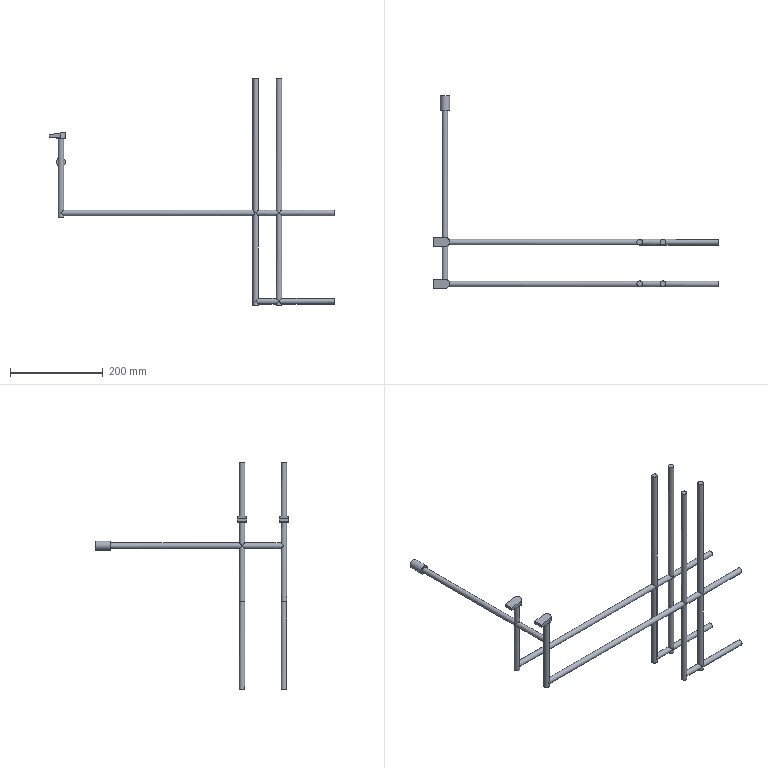Part | STEP file | solid 140 | 1 solid | 56 faces | box 614 x 415 x 490 mm | volume 485763 mm3 | cylinder 28 | plane 28 | commonest cylinder face diameters 12 x25 20 x3